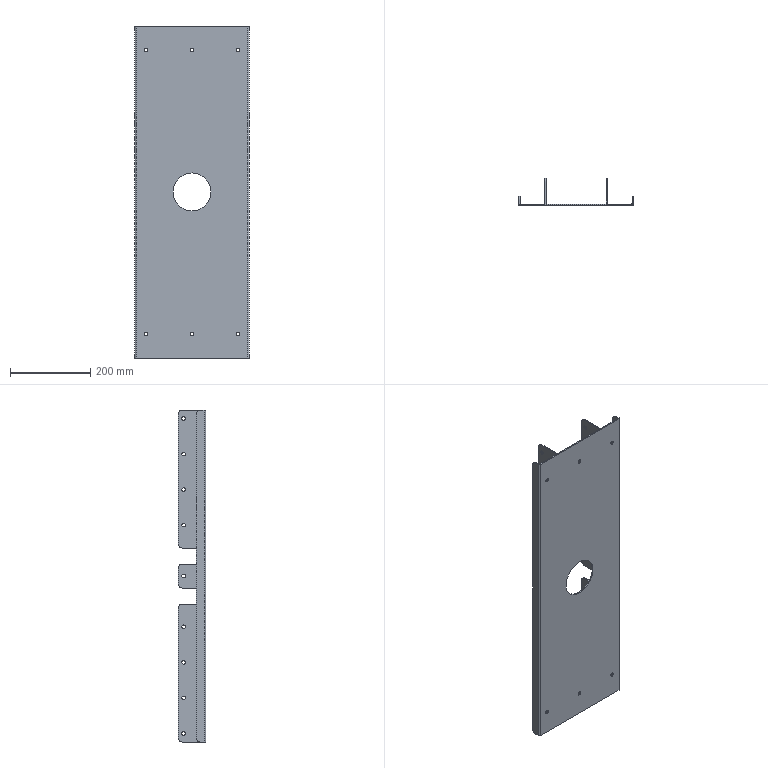Part | SolidWorks | features BaseBody 1 | 1 solid | 112 faces | box 286 x 68 x 830 mm | volume 1082690 mm3 | cylinder 70 | plane 42 | commonest cylinder face diameters 9 x48 20 x16 1 x2 7 x2 95 x2